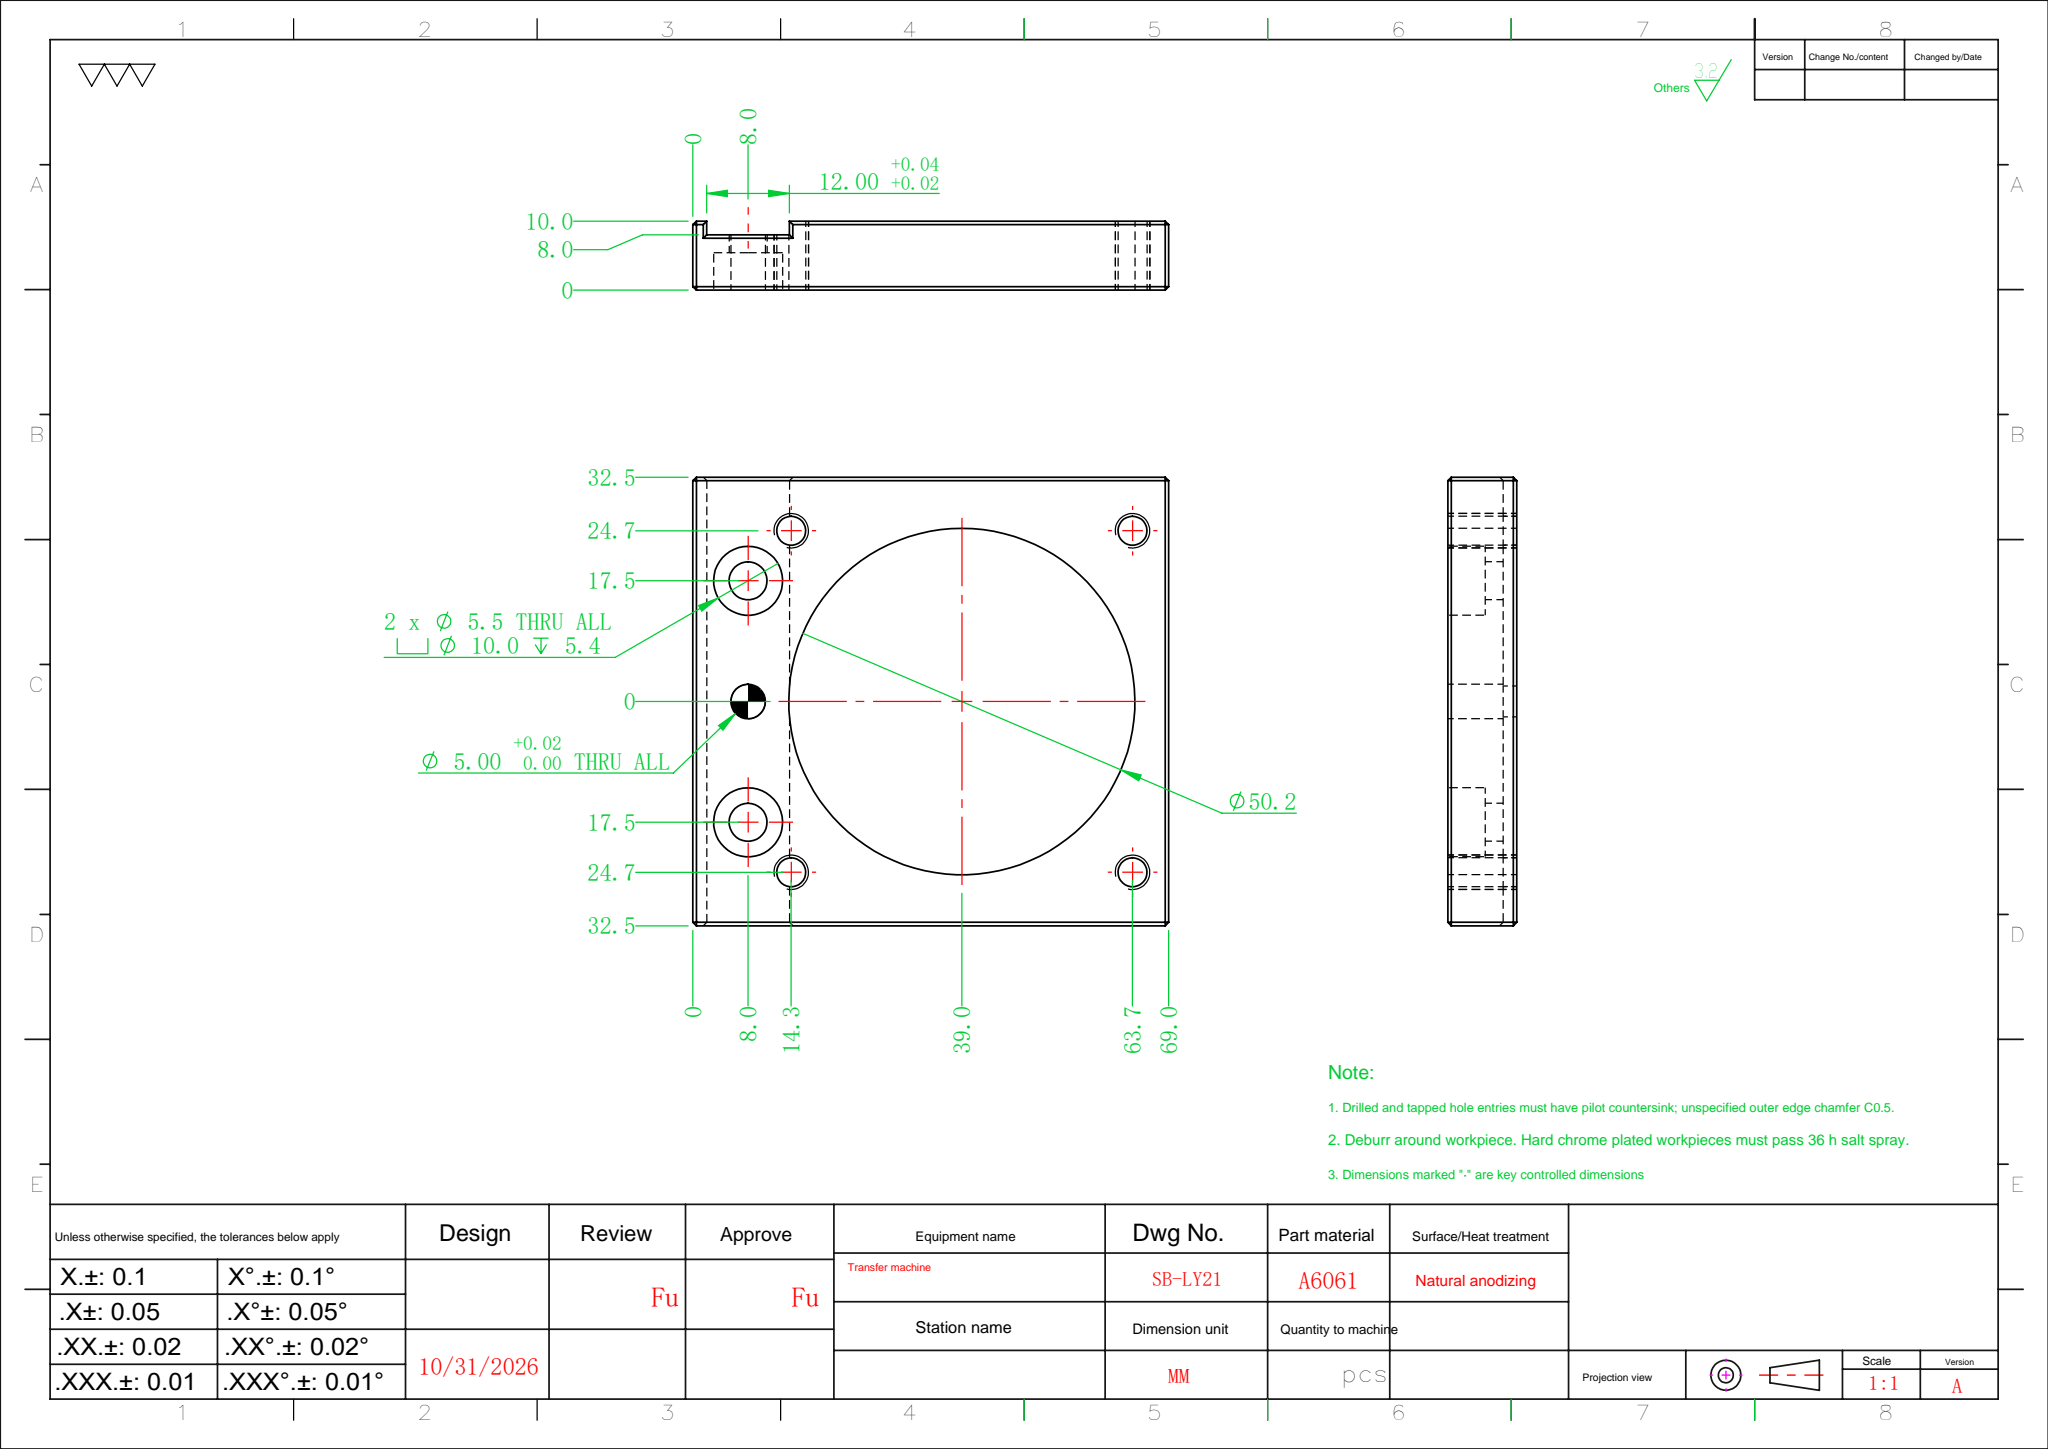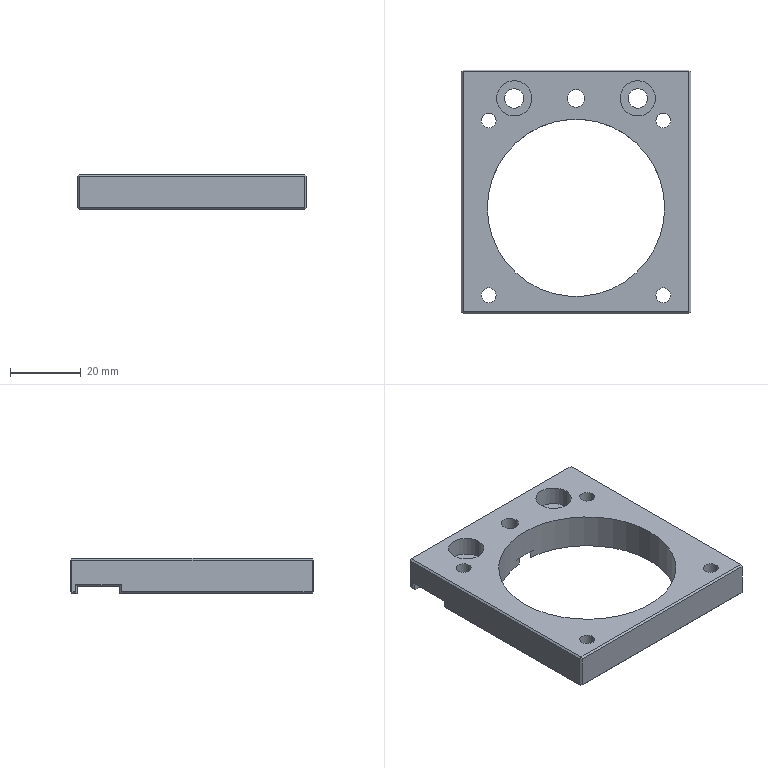Part | SolidWorks | features HoleWzd 3, Cut 2, Chamfer 1, Extrusion 1 | 1 solid | 63 faces | box 65 x 69 x 10 mm | volume 21766 mm3 | plane 43 | cylinder 20 | commonest cylinder face diameters 4.2 x8 5.5 x4 10 x4 5 x2 50.2 x2